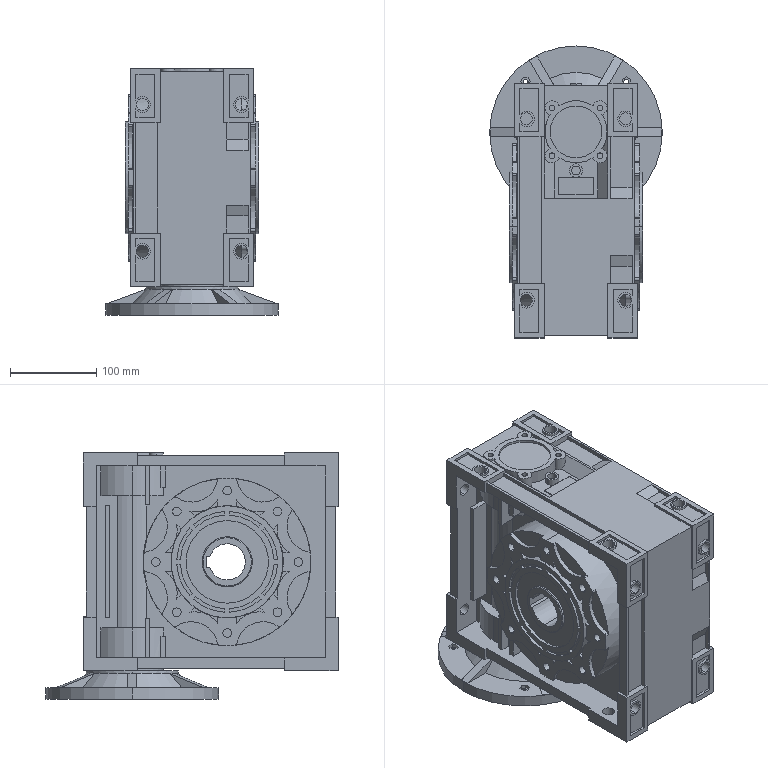Part | SolidWorks | features ICE 74, CirPattern 10, Chamfer 9, MirrorPattern 9, Revolution 5, DeleteBody 4, Fillet 3, MirrorSolid 2, Extrusion 1, LPattern 1, PLine 1, Rib 1 | 1 solid | 956 faces | box 200 x 338.5 x 285.25 mm | volume 8295656 mm3 | plane 613 | cylinder 315 | torus 16 | cone 12 | commonest cylinder face diameters 10 x48 61.845 x40 4.32 x36 18.2 x33 14 x28 108.68 x16